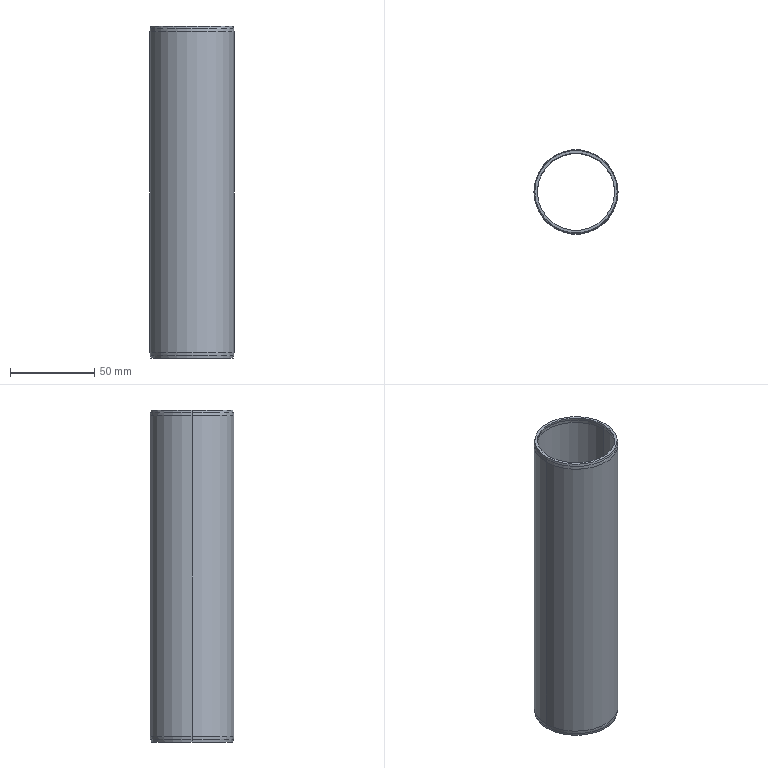Part | STEP file | 50x1.5B_1200-1 | 1 solid | 22 faces | box 50 x 50 x 197.6 mm | volume 45172 mm3 | spline 8 | cone 8 | cylinder 4 | plane 2 | commonest cylinder face diameters 47 x2 50 x2